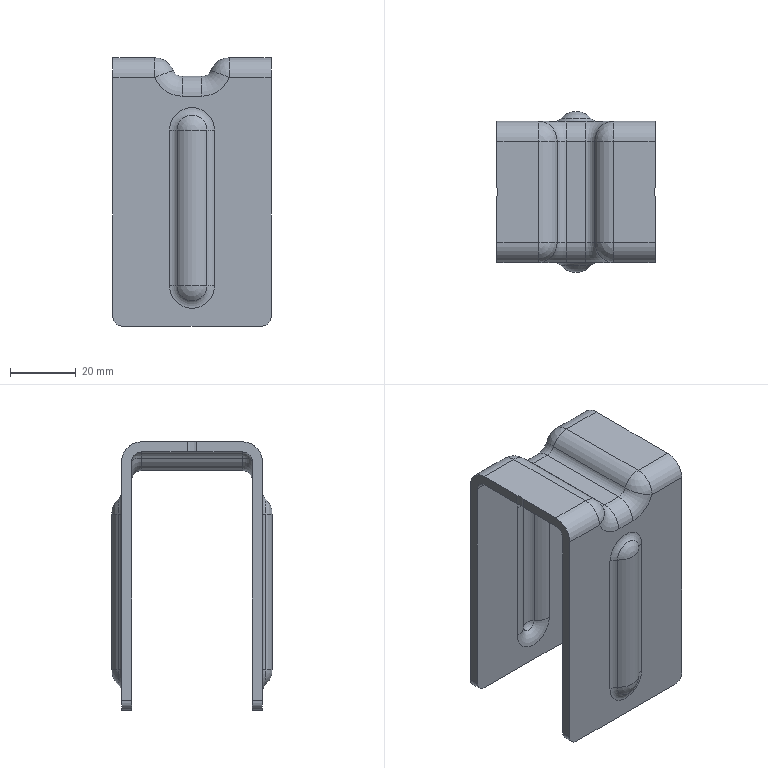Part | STEP file | PARTBODY_id314_x_t | 1 solid | 86 faces | box 48 x 48.7 x 81.415 mm | volume 29466 mm3 | cylinder 38 | plane 16 | sphere 16 | torus 16 | commonest cylinder face diameters 5.85 x10 12 x10 6.15 x6 12.3 x6 6 x4 9.576 x2